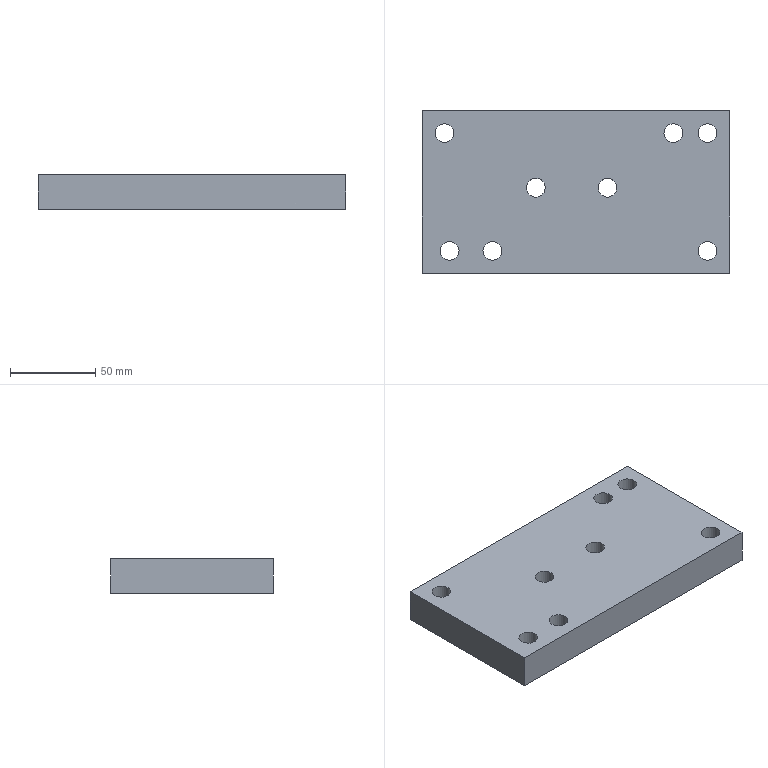Part | STEP file | 111_id2966_x_t | 1 solid | 14 faces | box 180 x 95 x 20 mm | volume 326795 mm3 | cylinder 8 | plane 6 | commonest cylinder face diameters 11 x8
STEP:
#1=CARTESIAN_POINT('',(0.,0.,0.));
#2=DIRECTION('',(0.,0.,1.));
#3=DIRECTION('',(1.,0.,0.));
#4=AXIS2_PLACEMENT_3D('',#1,#2,#3);
#5=CARTESIAN_POINT('',(638.481,67.,105.));
#6=VERTEX_POINT('',#5);
#7=CARTESIAN_POINT('',(627.481,67.,105.));
#8=VERTEX_POINT('',#7);
#9=CARTESIAN_POINT('',(632.981,67.,105.));
#10=DIRECTION('',(0.,0.,1.));
#11=DIRECTION('',(1.,0.,0.));
#12=AXIS2_PLACEMENT_3D('',#9,#10,#11);
#13=CIRCLE('',#12,5.5);
#14=CARTESIAN_POINT('',(657.5,68.,105.));
#15=DIRECTION('',(0.,0.,1.));
#16=DIRECTION('',(-1.,0.,0.));
#17=AXIS2_PLACEMENT_3D('',#14,#15,#16);
#18=PLANE('',#17);
#19=CARTESIAN_POINT('',(24.519,1.));
#20=DIRECTION('',(-1.,0.));
#21=AXIS2_PLACEMENT_2D('',#19,#20);
#22=CIRCLE('',#21,5.5);
#23=(GEOMETRIC_REPRESENTATION_CONTEXT(2)PARAMETRIC_REPRESENTATION_CONTEXT()REPRESENTATION_CONTEXT('',''));
#24=DEFINITIONAL_REPRESENTATION('',(#22),#23);
#25=PCURVE('',#18,#24);
#26=CARTESIAN_POINT('',(632.981,67.,-16.));
#27=DIRECTION('',(0.,0.,1.));
#28=DIRECTION('',(-1.,0.,0.));
#29=AXIS2_PLACEMENT_3D('',#26,#27,#28);
#30=CYLINDRICAL_SURFACE('',#29,5.5);
#31=CARTESIAN_POINT('',(3.142,121.));
#32=DIRECTION('',(1.,0.));
#33=VECTOR('',#32,1.);
#34=LINE('',#31,#33);
#35=(GEOMETRIC_REPRESENTATION_CONTEXT(2)PARAMETRIC_REPRESENTATION_CONTEXT()REPRESENTATION_CONTEXT('',''));
#36=DEFINITIONAL_REPRESENTATION('',(#34),#35);
#37=PCURVE('',#30,#36);
#38=SURFACE_CURVE('',#13,(#25,#37),.PCURVE_S1.);
#39=EDGE_CURVE('',#6,#8,#38,.T.);
#40=ORIENTED_EDGE('',*,*,#39,.F.);
#41=CARTESIAN_POINT('',(632.981,67.,105.));
#42=DIRECTION('',(0.,0.,1.));
#43=DIRECTION('',(1.,0.,0.));
#44=AXIS2_PLACEMENT_3D('',#41,#42,#43);
#45=CIRCLE('',#44,5.5);
#46=CARTESIAN_POINT('',(24.519,1.));
#47=DIRECTION('',(-1.,0.));
#48=AXIS2_PLACEMENT_2D('',#46,#47);
#49=CIRCLE('',#48,5.5);
#50=(GEOMETRIC_REPRESENTATION_CONTEXT(2)PARAMETRIC_REPRESENTATION_CONTEXT()REPRESENTATION_CONTEXT('',''));
#51=DEFINITIONAL_REPRESENTATION('',(#49),#50);
#52=PCURVE('',#18,#51);
#53=CARTESIAN_POINT('',(-3.142,121.));
#54=DIRECTION('',(1.,0.));
#55=VECTOR('',#54,1.);
#56=LINE('',#53,#55);
#57=(GEOMETRIC_REPRESENTATION_CONTEXT(2)PARAMETRIC_REPRESENTATION_CONTEXT()REPRESENTATION_CONTEXT('',''));
#58=DEFINITIONAL_REPRESENTATION('',(#56),#57);
#59=PCURVE('',#30,#58);
#60=SURFACE_CURVE('',#45,(#52,#59),.PCURVE_S1.);
#61=EDGE_CURVE('',#8,#6,#60,.T.);
#62=ORIENTED_EDGE('',*,*,#61,.F.);
#63=EDGE_LOOP('',(#40,#62));
#64=FACE_BOUND('',#63,.T.);
#65=CARTESIAN_POINT('',(680.481,67.,105.));
#66=VERTEX_POINT('',#65);
#67=CARTESIAN_POINT('',(674.981,67.,105.));
#68=DIRECTION('',(0.,0.,1.));
#69=DIRECTION('',(1.,0.,0.));
#70=AXIS2_PLACEMENT_3D('',#67,#68,#69);
#71=CIRCLE('',#70,5.5);
#72=CARTESIAN_POINT('',(-17.481,1.));
#73=DIRECTION('',(-1.,0.));
#74=AXIS2_PLACEMENT_2D('',#72,#73);
#75=CIRCLE('',#74,5.5);
#76=(GEOMETRIC_REPRESENTATION_CONTEXT(2)PARAMETRIC_REPRESENTATION_CONTEXT()REPRESENTATION_CONTEXT('',''));
#77=DEFINITIONAL_REPRESENTATION('',(#75),#76);
#78=PCURVE('',#18,#77);
#79=CARTESIAN_POINT('',(674.981,67.,-16.));
#80=DIRECTION('',(0.,0.,1.));
#81=DIRECTION('',(1.,0.,0.));
#82=AXIS2_PLACEMENT_3D('',#79,#80,#81);
#83=CYLINDRICAL_SURFACE('',#82,5.5);
#84=CARTESIAN_POINT('',(0.,121.));
#85=DIRECTION('',(1.,0.));
#86=VECTOR('',#85,1.);
#87=LINE('',#84,#86);
#88=(GEOMETRIC_REPRESENTATION_CONTEXT(2)PARAMETRIC_REPRESENTATION_CONTEXT()REPRESENTATION_CONTEXT('',''));
#89=DEFINITIONAL_REPRESENTATION('',(#87),#88);
#90=PCURVE('',#83,#89);
#91=SURFACE_CURVE('',#71,(#78,#90),.PCURVE_S1.);
#92=EDGE_CURVE('',#66,#66,#91,.T.);
#93=ORIENTED_EDGE('',*,*,#92,.F.);
#94=EDGE_LOOP('',(#93));
#95=FACE_BOUND('',#94,.T.);
#96=CARTESIAN_POINT('',(613.,30.,105.));
#97=VERTEX_POINT('',#96);
#98=CARTESIAN_POINT('',(607.5,30.,105.));
#99=DIRECTION('',(0.,0.,-1.));
#100=DIRECTION('',(1.,0.,0.));
#101=AXIS2_PLACEMENT_3D('',#98,#99,#100);
#102=CIRCLE('',#101,5.5);
#103=CARTESIAN_POINT('',(44.5,38.));
#104=CARTESIAN_POINT('',(44.5,47.526));
#105=CARTESIAN_POINT('',(52.75,42.763));
#106=CARTESIAN_POINT('',(61.,38.));
#107=CARTESIAN_POINT('',(52.75,33.237));
#108=CARTESIAN_POINT('',(44.5,28.474));
#109=CARTESIAN_POINT('',(44.5,38.));
#110=(BOUNDED_CURVE()B_SPLINE_CURVE(2,(#103,#104,#105,#106,#107,#108,#109),.UNSPECIFIED.,.T.,.F.)B_SPLINE_CURVE_WITH_KNOTS((1,2,2,2,2,1),(-2.094,0.,2.094,4.189,6.283,8.378),.UNSPECIFIED.)CURVE()GEOMETRIC_REPRESENTATION_ITEM()RATIONAL_B_SPLINE_CURVE((1.,0.5,1.,0.5,1.,0.5,1.))REPRESENTATION_ITEM(''));
#111=(GEOMETRIC_REPRESENTATION_CONTEXT(2)PARAMETRIC_REPRESENTATION_CONTEXT()REPRESENTATION_CONTEXT('',''));
#112=DEFINITIONAL_REPRESENTATION('',(#110),#111);
#113=PCURVE('',#18,#112);
#114=CARTESIAN_POINT('',(607.5,30.,90.));
#115=DIRECTION('',(0.,0.,1.));
#116=DIRECTION('',(-1.,0.,0.));
#117=AXIS2_PLACEMENT_3D('',#114,#115,#116);
#118=CYLINDRICAL_SURFACE('',#117,5.5);
#119=CARTESIAN_POINT('',(9.425,15.));
#120=DIRECTION('',(-1.,0.));
#121=VECTOR('',#120,1.);
#122=LINE('',#119,#121);
#123=(GEOMETRIC_REPRESENTATION_CONTEXT(2)PARAMETRIC_REPRESENTATION_CONTEXT()REPRESENTATION_CONTEXT('',''));
#124=DEFINITIONAL_REPRESENTATION('',(#122),#123);
#125=PCURVE('',#118,#124);
#126=SURFACE_CURVE('',#102,(#113,#125),.PCURVE_S1.);
#127=EDGE_CURVE('',#97,#97,#126,.T.);
#128=ORIENTED_EDGE('',*,*,#127,.T.);
#129=EDGE_LOOP('',(#128));
#130=FACE_BOUND('',#129,.T.);
#131=CARTESIAN_POINT('',(739.,99.,105.));
#132=VERTEX_POINT('',#131);
#133=CARTESIAN_POINT('',(733.5,99.,105.));
#134=DIRECTION('',(0.,0.,-1.));
#135=DIRECTION('',(1.,0.,0.));
#136=AXIS2_PLACEMENT_3D('',#133,#134,#135);
#137=CIRCLE('',#136,5.5);
#138=CARTESIAN_POINT('',(-81.5,-31.));
#139=CARTESIAN_POINT('',(-81.5,-21.474));
#140=CARTESIAN_POINT('',(-73.25,-26.237));
#141=CARTESIAN_POINT('',(-65.,-31.));
#142=CARTESIAN_POINT('',(-73.25,-35.763));
#143=CARTESIAN_POINT('',(-81.5,-40.526));
#144=CARTESIAN_POINT('',(-81.5,-31.));
#145=(BOUNDED_CURVE()B_SPLINE_CURVE(2,(#138,#139,#140,#141,#142,#143,#144),.UNSPECIFIED.,.T.,.F.)B_SPLINE_CURVE_WITH_KNOTS((1,2,2,2,2,1),(-2.094,0.,2.094,4.189,6.283,8.378),.UNSPECIFIED.)CURVE()GEOMETRIC_REPRESENTATION_ITEM()RATIONAL_B_SPLINE_CURVE((1.,0.5,1.,0.5,1.,0.5,1.))REPRESENTATION_ITEM(''));
#146=(GEOMETRIC_REPRESENTATION_CONTEXT(2)PARAMETRIC_REPRESENTATION_CONTEXT()REPRESENTATION_CONTEXT('',''));
#147=DEFINITIONAL_REPRESENTATION('',(#145),#146);
#148=PCURVE('',#18,#147);
#149=CARTESIAN_POINT('',(733.5,99.,90.));
#150=DIRECTION('',(0.,0.,1.));
#151=DIRECTION('',(-1.,0.,0.));
#152=AXIS2_PLACEMENT_3D('',#149,#150,#151);
#153=CYLINDRICAL_SURFACE('',#152,5.5);
#154=CARTESIAN_POINT('',(9.425,15.));
#155=DIRECTION('',(-1.,0.));
#156=VECTOR('',#155,1.);
#157=LINE('',#154,#156);
#158=(GEOMETRIC_REPRESENTATION_CONTEXT(2)PARAMETRIC_REPRESENTATION_CONTEXT()REPRESENTATION_CONTEXT('',''));
#159=DEFINITIONAL_REPRESENTATION('',(#157),#158);
#160=PCURVE('',#153,#159);
#161=SURFACE_CURVE('',#137,(#148,#160),.PCURVE_S1.);
#162=EDGE_CURVE('',#132,#132,#161,.T.);
#163=ORIENTED_EDGE('',*,*,#162,.T.);
#164=EDGE_LOOP('',(#163));
#165=FACE_BOUND('',#164,.T.);
#166=CARTESIAN_POINT('',(588.,30.,105.));
#167=VERTEX_POINT('',#166);
#168=CARTESIAN_POINT('',(582.5,30.,105.));
#169=DIRECTION('',(0.,0.,-1.));
#170=DIRECTION('',(1.,0.,0.));
#171=AXIS2_PLACEMENT_3D('',#168,#169,#170);
#172=CIRCLE('',#171,5.5);
#173=CARTESIAN_POINT('',(69.5,38.));
#174=CARTESIAN_POINT('',(69.5,47.526));
#175=CARTESIAN_POINT('',(77.75,42.763));
#176=CARTESIAN_POINT('',(86.,38.));
#177=CARTESIAN_POINT('',(77.75,33.237));
#178=CARTESIAN_POINT('',(69.5,28.474));
#179=CARTESIAN_POINT('',(69.5,38.));
#180=(BOUNDED_CURVE()B_SPLINE_CURVE(2,(#173,#174,#175,#176,#177,#178,#179),.UNSPECIFIED.,.T.,.F.)B_SPLINE_CURVE_WITH_KNOTS((1,2,2,2,2,1),(-2.094,0.,2.094,4.189,6.283,8.378),.UNSPECIFIED.)CURVE()GEOMETRIC_REPRESENTATION_ITEM()RATIONAL_B_SPLINE_CURVE((1.,0.5,1.,0.5,1.,0.5,1.))REPRESENTATION_ITEM(''));
#181=(GEOMETRIC_REPRESENTATION_CONTEXT(2)PARAMETRIC_REPRESENTATION_CONTEXT()REPRESENTATION_CONTEXT('',''));
#182=DEFINITIONAL_REPRESENTATION('',(#180),#181);
#183=PCURVE('',#18,#182);
#184=CARTESIAN_POINT('',(582.5,30.,90.));
#185=DIRECTION('',(0.,0.,1.));
#186=DIRECTION('',(-1.,0.,0.));
#187=AXIS2_PLACEMENT_3D('',#184,#185,#186);
#188=CYLINDRICAL_SURFACE('',#187,5.5);
#189=CARTESIAN_POINT('',(9.425,15.));
#190=DIRECTION('',(-1.,0.));
#191=VECTOR('',#190,1.);
#192=LINE('',#189,#191);
#193=(GEOMETRIC_REPRESENTATION_CONTEXT(2)PARAMETRIC_REPRESENTATION_CONTEXT()REPRESENTATION_CONTEXT('',''));
#194=DEFINITIONAL_REPRESENTATION('',(#192),#193);
#195=PCURVE('',#188,#194);
#196=SURFACE_CURVE('',#172,(#183,#195),.PCURVE_S1.);
#197=EDGE_CURVE('',#167,#167,#196,.T.);
#198=ORIENTED_EDGE('',*,*,#197,.T.);
#199=EDGE_LOOP('',(#198));
#200=FACE_BOUND('',#199,.T.);
#201=CARTESIAN_POINT('',(746.5,17.,105.));
#202=VERTEX_POINT('',#201);
#203=CARTESIAN_POINT('',(566.5,17.,105.));
#204=VERTEX_POINT('',#203);
#205=CARTESIAN_POINT('',(657.5,17.,105.));
#206=DIRECTION('',(-1.,0.,0.));
#207=VECTOR('',#206,1.);
#208=LINE('',#205,#207);
#209=CARTESIAN_POINT('',(0.,51.));
#210=DIRECTION('',(1.,0.));
#211=VECTOR('',#210,1.);
#212=LINE('',#209,#211);
#213=(GEOMETRIC_REPRESENTATION_CONTEXT(2)PARAMETRIC_REPRESENTATION_CONTEXT()REPRESENTATION_CONTEXT('',''));
#214=DEFINITIONAL_REPRESENTATION('',(#212),#213);
#215=PCURVE('',#18,#214);
#216=CARTESIAN_POINT('',(657.5,17.,90.));
#217=DIRECTION('',(0.,-1.,0.));
#218=DIRECTION('',(0.,0.,1.));
#219=AXIS2_PLACEMENT_3D('',#216,#217,#218);
#220=PLANE('',#219);
#221=CARTESIAN_POINT('',(15.,0.));
#222=DIRECTION('',(0.,1.));
#223=VECTOR('',#222,1.);
#224=LINE('',#221,#223);
#225=(GEOMETRIC_REPRESENTATION_CONTEXT(2)PARAMETRIC_REPRESENTATION_CONTEXT()REPRESENTATION_CONTEXT('',''));
#226=DEFINITIONAL_REPRESENTATION('',(#224),#225);
#227=PCURVE('',#220,#226);
#228=SURFACE_CURVE('',#208,(#215,#227),.PCURVE_S1.);
#229=EDGE_CURVE('',#202,#204,#228,.T.);
#230=ORIENTED_EDGE('',*,*,#229,.F.);
#231=CARTESIAN_POINT('',(746.5,112.,105.));
#232=VERTEX_POINT('',#231);
#233=CARTESIAN_POINT('',(746.5,68.,105.));
#234=DIRECTION('',(0.,-1.,0.));
#235=VECTOR('',#234,1.);
#236=LINE('',#233,#235);
#237=CARTESIAN_POINT('',(-89.,0.));
#238=DIRECTION('',(0.,1.));
#239=VECTOR('',#238,1.);
#240=LINE('',#237,#239);
#241=(GEOMETRIC_REPRESENTATION_CONTEXT(2)PARAMETRIC_REPRESENTATION_CONTEXT()REPRESENTATION_CONTEXT('',''));
#242=DEFINITIONAL_REPRESENTATION('',(#240),#241);
#243=PCURVE('',#18,#242);
#244=CARTESIAN_POINT('',(746.5,68.,90.));
#245=DIRECTION('',(1.,0.,0.));
#246=DIRECTION('',(0.,0.,1.));
#247=AXIS2_PLACEMENT_3D('',#244,#245,#246);
#248=PLANE('',#247);
#249=CARTESIAN_POINT('',(15.,0.));
#250=DIRECTION('',(0.,1.));
#251=VECTOR('',#250,1.);
#252=LINE('',#249,#251);
#253=(GEOMETRIC_REPRESENTATION_CONTEXT(2)PARAMETRIC_REPRESENTATION_CONTEXT()REPRESENTATION_CONTEXT('',''));
#254=DEFINITIONAL_REPRESENTATION('',(#252),#253);
#255=PCURVE('',#248,#254);
#256=SURFACE_CURVE('',#236,(#243,#255),.PCURVE_S1.);
#257=EDGE_CURVE('',#232,#202,#256,.T.);
#258=ORIENTED_EDGE('',*,*,#257,.F.);
#259=CARTESIAN_POINT('',(566.5,112.,105.));
#260=VERTEX_POINT('',#259);
#261=CARTESIAN_POINT('',(657.5,112.,105.));
#262=DIRECTION('',(1.,0.,0.));
#263=VECTOR('',#262,1.);
#264=LINE('',#261,#263);
#265=CARTESIAN_POINT('',(0.,-44.));
#266=DIRECTION('',(-1.,0.));
#267=VECTOR('',#266,1.);
#268=LINE('',#265,#267);
#269=(GEOMETRIC_REPRESENTATION_CONTEXT(2)PARAMETRIC_REPRESENTATION_CONTEXT()REPRESENTATION_CONTEXT('',''));
#270=DEFINITIONAL_REPRESENTATION('',(#268),#269);
#271=PCURVE('',#18,#270);
#272=CARTESIAN_POINT('',(657.5,112.,90.));
#273=DIRECTION('',(0.,1.,0.));
#274=DIRECTION('',(0.,0.,-1.));
#275=AXIS2_PLACEMENT_3D('',#272,#273,#274);
#276=PLANE('',#275);
#277=CARTESIAN_POINT('',(-15.,0.));
#278=DIRECTION('',(0.,-1.));
#279=VECTOR('',#278,1.);
#280=LINE('',#277,#279);
#281=(GEOMETRIC_REPRESENTATION_CONTEXT(2)PARAMETRIC_REPRESENTATION_CONTEXT()REPRESENTATION_CONTEXT('',''));
#282=DEFINITIONAL_REPRESENTATION('',(#280),#281);
#283=PCURVE('',#276,#282);
#284=SURFACE_CURVE('',#264,(#271,#283),.PCURVE_S1.);
#285=EDGE_CURVE('',#260,#232,#284,.T.);
#286=ORIENTED_EDGE('',*,*,#285,.F.);
#287=CARTESIAN_POINT('',(566.5,68.,105.));
#288=DIRECTION('',(0.,1.,0.));
#289=VECTOR('',#288,1.);
#290=LINE('',#287,#289);
#291=CARTESIAN_POINT('',(91.,0.));
#292=DIRECTION('',(0.,-1.));
#293=VECTOR('',#292,1.);
#294=LINE('',#291,#293);
#295=(GEOMETRIC_REPRESENTATION_CONTEXT(2)PARAMETRIC_REPRESENTATION_CONTEXT()REPRESENTATION_CONTEXT('',''));
#296=DEFINITIONAL_REPRESENTATION('',(#294),#295);
#297=PCURVE('',#18,#296);
#298=CARTESIAN_POINT('',(566.5,68.,90.));
#299=DIRECTION('',(-1.,0.,0.));
#300=DIRECTION('',(0.,0.,-1.));
#301=AXIS2_PLACEMENT_3D('',#298,#299,#300);
#302=PLANE('',#301);
#303=CARTESIAN_POINT('',(-15.,0.));
#304=DIRECTION('',(0.,-1.));
#305=VECTOR('',#304,1.);
#306=LINE('',#303,#305);
#307=(GEOMETRIC_REPRESENTATION_CONTEXT(2)PARAMETRIC_REPRESENTATION_CONTEXT()REPRESENTATION_CONTEXT('',''));
#308=DEFINITIONAL_REPRESENTATION('',(#306),#307);
#309=PCURVE('',#302,#308);
#310=SURFACE_CURVE('',#290,(#297,#309),.PCURVE_S1.);
#311=EDGE_CURVE('',#204,#260,#310,.T.);
#312=ORIENTED_EDGE('',*,*,#311,.F.);
#313=EDGE_LOOP('',(#230,#258,#286,#312));
#314=FACE_BOUND('',#313,.T.);
#315=CARTESIAN_POINT('',(739.,30.,105.));
#316=VERTEX_POINT('',#315);
#317=CARTESIAN_POINT('',(733.5,30.,105.));
#318=DIRECTION('',(0.,0.,-1.));
#319=DIRECTION('',(1.,0.,0.));
#320=AXIS2_PLACEMENT_3D('',#317,#318,#319);
#321=CIRCLE('',#320,5.5);
#322=CARTESIAN_POINT('',(-81.5,38.));
#323=CARTESIAN_POINT('',(-81.5,47.526));
#324=CARTESIAN_POINT('',(-73.25,42.763));
#325=CARTESIAN_POINT('',(-65.,38.));
#326=CARTESIAN_POINT('',(-73.25,33.237));
#327=CARTESIAN_POINT('',(-81.5,28.474));
#328=CARTESIAN_POINT('',(-81.5,38.));
#329=(BOUNDED_CURVE()B_SPLINE_CURVE(2,(#322,#323,#324,#325,#326,#327,#328),.UNSPECIFIED.,.T.,.F.)B_SPLINE_CURVE_WITH_KNOTS((1,2,2,2,2,1),(-2.094,0.,2.094,4.189,6.283,8.378),.UNSPECIFIED.)CURVE()GEOMETRIC_REPRESENTATION_ITEM()RATIONAL_B_SPLINE_CURVE((1.,0.5,1.,0.5,1.,0.5,1.))REPRESENTATION_ITEM(''));
#330=(GEOMETRIC_REPRESENTATION_CONTEXT(2)PARAMETRIC_REPRESENTATION_CONTEXT()REPRESENTATION_CONTEXT('',''));
#331=DEFINITIONAL_REPRESENTATION('',(#329),#330);
#332=PCURVE('',#18,#331);
#333=CARTESIAN_POINT('',(733.5,30.,90.));
#334=DIRECTION('',(0.,0.,1.));
#335=DIRECTION('',(-1.,0.,0.));
#336=AXIS2_PLACEMENT_3D('',#333,#334,#335);
#337=CYLINDRICAL_SURFACE('',#336,5.5);
#338=CARTESIAN_POINT('',(9.425,15.));
#339=DIRECTION('',(-1.,0.));
#340=VECTOR('',#339,1.);
#341=LINE('',#338,#340);
#342=(GEOMETRIC_REPRESENTATION_CONTEXT(2)PARAMETRIC_REPRESENTATION_CONTEXT()REPRESENTATION_CONTEXT('',''));
#343=DEFINITIONAL_REPRESENTATION('',(#341),#342);
#344=PCURVE('',#337,#343);
#345=SURFACE_CURVE('',#321,(#332,#344),.PCURVE_S1.);
#346=EDGE_CURVE('',#316,#316,#345,.T.);
#347=ORIENTED_EDGE('',*,*,#346,.T.);
#348=EDGE_LOOP('',(#347));
#349=FACE_BOUND('',#348,.T.);
#350=CARTESIAN_POINT('',(585.,99.,105.));
#351=VERTEX_POINT('',#350);
#352=CARTESIAN_POINT('',(579.5,99.,105.));
#353=DIRECTION('',(0.,0.,-1.));
#354=DIRECTION('',(1.,0.,0.));
#355=AXIS2_PLACEMENT_3D('',#352,#353,#354);
#356=CIRCLE('',#355,5.5);
#357=CARTESIAN_POINT('',(72.5,-31.));
#358=CARTESIAN_POINT('',(72.5,-21.474));
#359=CARTESIAN_POINT('',(80.75,-26.237));
#360=CARTESIAN_POINT('',(89.,-31.));
#361=CARTESIAN_POINT('',(80.75,-35.763));
#362=CARTESIAN_POINT('',(72.5,-40.526));
#363=CARTESIAN_POINT('',(72.5,-31.));
#364=(BOUNDED_CURVE()B_SPLINE_CURVE(2,(#357,#358,#359,#360,#361,#362,#363),.UNSPECIFIED.,.T.,.F.)B_SPLINE_CURVE_WITH_KNOTS((1,2,2,2,2,1),(-2.094,0.,2.094,4.189,6.283,8.378),.UNSPECIFIED.)CURVE()GEOMETRIC_REPRESENTATION_ITEM()RATIONAL_B_SPLINE_CURVE((1.,0.5,1.,0.5,1.,0.5,1.))REPRESENTATION_ITEM(''));
#365=(GEOMETRIC_REPRESENTATION_CONTEXT(2)PARAMETRIC_REPRESENTATION_CONTEXT()REPRESENTATION_CONTEXT('',''));
#366=DEFINITIONAL_REPRESENTATION('',(#364),#365);
#367=PCURVE('',#18,#366);
#368=CARTESIAN_POINT('',(579.5,99.,90.));
#369=DIRECTION('',(0.,0.,1.));
#370=DIRECTION('',(-1.,0.,0.));
#371=AXIS2_PLACEMENT_3D('',#368,#369,#370);
#372=CYLINDRICAL_SURFACE('',#371,5.5);
#373=CARTESIAN_POINT('',(9.425,15.));
#374=DIRECTION('',(-1.,0.));
#375=VECTOR('',#374,1.);
#376=LINE('',#373,#375);
#377=(GEOMETRIC_REPRESENTATION_CONTEXT(2)PARAMETRIC_REPRESENTATION_CONTEXT()REPRESENTATION_CONTEXT('',''));
#378=DEFINITIONAL_REPRESENTATION('',(#376),#377);
#379=PCURVE('',#372,#378);
#380=SURFACE_CURVE('',#356,(#367,#379),.PCURVE_S1.);
#381=EDGE_CURVE('',#351,#351,#380,.T.);
#382=ORIENTED_EDGE('',*,*,#381,.T.);
#383=EDGE_LOOP('',(#382));
#384=FACE_BOUND('',#383,.T.);
#385=CARTESIAN_POINT('',(719.,99.,105.));
#386=VERTEX_POINT('',#385);
#387=CARTESIAN_POINT('',(713.5,99.,105.));
#388=DIRECTION('',(0.,0.,-1.));
#389=DIRECTION('',(1.,0.,0.));
#390=AXIS2_PLACEMENT_3D('',#387,#388,#389);
#391=CIRCLE('',#390,5.5);
#392=CARTESIAN_POINT('',(-61.5,-31.));
#393=CARTESIAN_POINT('',(-61.5,-21.474));
#394=CARTESIAN_POINT('',(-53.25,-26.237));
#395=CARTESIAN_POINT('',(-45.,-31.));
#396=CARTESIAN_POINT('',(-53.25,-35.763));
#397=CARTESIAN_POINT('',(-61.5,-40.526));
#398=CARTESIAN_POINT('',(-61.5,-31.));
#399=(BOUNDED_CURVE()B_SPLINE_CURVE(2,(#392,#393,#394,#395,#396,#397,#398),.UNSPECIFIED.,.T.,.F.)B_SPLINE_CURVE_WITH_KNOTS((1,2,2,2,2,1),(-2.094,0.,2.094,4.189,6.283,8.378),.UNSPECIFIED.)CURVE()GEOMETRIC_REPRESENTATION_ITEM()RATIONAL_B_SPLINE_CURVE((1.,0.5,1.,0.5,1.,0.5,1.))REPRESENTATION_ITEM(''));
#400=(GEOMETRIC_REPRESENTATION_CONTEXT(2)PARAMETRIC_REPRESENTATION_CONTEXT()REPRESENTATION_CONTEXT('',''));
#401=DEFINITIONAL_REPRESENTATION('',(#399),#400);
#402=PCURVE('',#18,#401);
#403=CARTESIAN_POINT('',(713.5,99.,90.));
#404=DIRECTION('',(0.,0.,1.));
#405=DIRECTION('',(-1.,0.,0.));
#406=AXIS2_PLACEMENT_3D('',#403,#404,#405);
#407=CYLINDRICAL_SURFACE('',#406,5.5);
#408=CARTESIAN_POINT('',(9.425,15.));
#409=DIRECTION('',(-1.,0.));
#410=VECTOR('',#409,1.);
#411=LINE('',#408,#410);
#412=(GEOMETRIC_REPRESENTATION_CONTEXT(2)PARAMETRIC_REPRESENTATION_CONTEXT()REPRESENTATION_CONTEXT('',''));
#413=DEFINITIONAL_REPRESENTATION('',(#411),#412);
#414=PCURVE('',#407,#413);
#415=SURFACE_CURVE('',#391,(#402,#414),.PCURVE_S1.);
#416=EDGE_CURVE('',#386,#386,#415,.T.);
#417=ORIENTED_EDGE('',*,*,#416,.T.);
#418=EDGE_LOOP('',(#417));
#419=FACE_BOUND('',#418,.T.);
#420=ADVANCED_FACE('',(#64,#95,#130,#165,#200,#314,#349,#384,#419),#18,.T.);
#421=CARTESIAN_POINT('',(627.481,67.,85.));
#422=VERTEX_POINT('',#421);
#423=CARTESIAN_POINT('',(632.981,67.,85.));
#424=DIRECTION('',(0.,0.,-1.));
#425=DIRECTION('',(-1.,0.,0.));
#426=AXIS2_PLACEMENT_3D('',#423,#424,#425);
#427=CIRCLE('',#426,5.5);
#428=CARTESIAN_POINT('',(657.5,68.,85.));
#429=DIRECTION('',(0.,0.,-1.));
#430=DIRECTION('',(1.,0.,0.));
#431=AXIS2_PLACEMENT_3D('',#428,#429,#430);
#432=PLANE('',#431);
#433=CARTESIAN_POINT('',(-24.519,1.));
#434=DIRECTION('',(-1.,0.));
#435=AXIS2_PLACEMENT_2D('',#433,#434);
#436=CIRCLE('',#435,5.5);
#437=(GEOMETRIC_REPRESENTATION_CONTEXT(2)PARAMETRIC_REPRESENTATION_CONTEXT()REPRESENTATION_CONTEXT('',''));
#438=DEFINITIONAL_REPRESENTATION('',(#436),#437);
#439=PCURVE('',#432,#438);
#440=CARTESIAN_POINT('',(6.283,101.));
#441=DIRECTION('',(-1.,0.));
#442=VECTOR('',#441,1.);
#443=LINE('',#440,#442);
#444=(GEOMETRIC_REPRESENTATION_CONTEXT(2)PARAMETRIC_REPRESENTATION_CONTEXT()REPRESENTATION_CONTEXT('',''));
#445=DEFINITIONAL_REPRESENTATION('',(#443),#444);
#446=PCURVE('',#30,#445);
#447=SURFACE_CURVE('',#427,(#439,#446),.PCURVE_S1.);
#448=EDGE_CURVE('',#422,#422,#447,.T.);
#449=ORIENTED_EDGE('',*,*,#448,.F.);
#450=EDGE_LOOP('',(#449));
#451=FACE_BOUND('',#450,.T.);
#452=CARTESIAN_POINT('',(669.481,67.,85.));
#453=VERTEX_POINT('',#452);
#454=CARTESIAN_POINT('',(680.481,67.,85.));
#455=VERTEX_POINT('',#454);
#456=CARTESIAN_POINT('',(674.981,67.,85.));
#457=DIRECTION('',(0.,0.,-1.));
#458=DIRECTION('',(-1.,0.,0.));
#459=AXIS2_PLACEMENT_3D('',#456,#457,#458);
#460=CIRCLE('',#459,5.5);
#461=CARTESIAN_POINT('',(17.481,1.));
#462=DIRECTION('',(-1.,0.));
#463=AXIS2_PLACEMENT_2D('',#461,#462);
#464=CIRCLE('',#463,5.5);
#465=(GEOMETRIC_REPRESENTATION_CONTEXT(2)PARAMETRIC_REPRESENTATION_CONTEXT()REPRESENTATION_CONTEXT('',''));
#466=DEFINITIONAL_REPRESENTATION('',(#464),#465);
#467=PCURVE('',#432,#466);
#468=CARTESIAN_POINT('',(3.142,101.));
#469=DIRECTION('',(-1.,0.));
#470=VECTOR('',#469,1.);
#471=LINE('',#468,#470);
#472=(GEOMETRIC_REPRESENTATION_CONTEXT(2)PARAMETRIC_REPRESENTATION_CONTEXT()REPRESENTATION_CONTEXT('',''));
#473=DEFINITIONAL_REPRESENTATION('',(#471),#472);
#474=PCURVE('',#83,#473);
#475=SURFACE_CURVE('',#460,(#467,#474),.PCURVE_S1.);
#476=EDGE_CURVE('',#453,#455,#475,.T.);
#477=ORIENTED_EDGE('',*,*,#476,.F.);
#478=CARTESIAN_POINT('',(674.981,67.,85.));
#479=DIRECTION('',(0.,0.,-1.));
#480=DIRECTION('',(-1.,0.,0.));
#481=AXIS2_PLACEMENT_3D('',#478,#479,#480);
#482=CIRCLE('',#481,5.5);
#483=CARTESIAN_POINT('',(17.481,1.));
#484=DIRECTION('',(-1.,0.));
#485=AXIS2_PLACEMENT_2D('',#483,#484);
#486=CIRCLE('',#485,5.5);
#487=(GEOMETRIC_REPRESENTATION_CONTEXT(2)PARAMETRIC_REPRESENTATION_CONTEXT()REPRESENTATION_CONTEXT('',''));
#488=DEFINITIONAL_REPRESENTATION('',(#486),#487);
#489=PCURVE('',#432,#488);
#490=CARTESIAN_POINT('',(9.425,101.));
#491=DIRECTION('',(-1.,0.));
#492=VECTOR('',#491,1.);
#493=LINE('',#490,#492);
#494=(GEOMETRIC_REPRESENTATION_CONTEXT(2)PARAMETRIC_REPRESENTATION_CONTEXT()REPRESENTATION_CONTEXT('',''));
#495=DEFINITIONAL_REPRESENTATION('',(#493),#494);
#496=PCURVE('',#83,#495);
#497=SURFACE_CURVE('',#482,(#489,#496),.PCURVE_S1.);
#498=EDGE_CURVE('',#455,#453,#497,.T.);
#499=ORIENTED_EDGE('',*,*,#498,.F.);
#500=EDGE_LOOP('',(#477,#499));
#501=FACE_BOUND('',#500,.T.);
#502=CARTESIAN_POINT('',(613.,30.,85.));
#503=VERTEX_POINT('',#502);
#504=CARTESIAN_POINT('',(607.5,30.,85.));
#505=DIRECTION('',(0.,0.,1.));
#506=DIRECTION('',(-1.,0.,0.));
#507=AXIS2_PLACEMENT_3D('',#504,#505,#506);
#508=CIRCLE('',#507,5.5);
#509=CARTESIAN_POINT('',(-55.5,38.));
#510=CARTESIAN_POINT('',(-55.5,47.526));
#511=CARTESIAN_POINT('',(-47.25,42.763));
#512=CARTESIAN_POINT('',(-39.,38.));
#513=CARTESIAN_POINT('',(-47.25,33.237));
#514=CARTESIAN_POINT('',(-55.5,28.474));
#515=CARTESIAN_POINT('',(-55.5,38.));
#516=(BOUNDED_CURVE()B_SPLINE_CURVE(2,(#509,#510,#511,#512,#513,#514,#515),.UNSPECIFIED.,.T.,.F.)B_SPLINE_CURVE_WITH_KNOTS((1,2,2,2,2,1),(-2.094,0.,2.094,4.189,6.283,8.378),.UNSPECIFIED.)CURVE()GEOMETRIC_REPRESENTATION_ITEM()RATIONAL_B_SPLINE_CURVE((1.,0.5,1.,0.5,1.,0.5,1.))REPRESENTATION_ITEM(''));
#517=(GEOMETRIC_REPRESENTATION_CONTEXT(2)PARAMETRIC_REPRESENTATION_CONTEXT()REPRESENTATION_CONTEXT('',''));
#518=DEFINITIONAL_REPRESENTATION('',(#516),#517);
#519=PCURVE('',#432,#518);
#520=CARTESIAN_POINT('',(0.,-5.));
#521=DIRECTION('',(1.,0.));
#522=VECTOR('',#521,1.);
#523=LINE('',#520,#522);
#524=(GEOMETRIC_REPRESENTATION_CONTEXT(2)PARAMETRIC_REPRESENTATION_CONTEXT()REPRESENTATION_CONTEXT('',''));
#525=DEFINITIONAL_REPRESENTATION('',(#523),#524);
#526=PCURVE('',#118,#525);
#527=SURFACE_CURVE('',#508,(#519,#526),.PCURVE_S1.);
#528=EDGE_CURVE('',#503,#503,#527,.T.);
#529=ORIENTED_EDGE('',*,*,#528,.T.);
#530=EDGE_LOOP('',(#529));
#531=FACE_BOUND('',#530,.T.);
#532=CARTESIAN_POINT('',(739.,99.,85.));
#533=VERTEX_POINT('',#532);
#534=CARTESIAN_POINT('',(733.5,99.,85.));
#535=DIRECTION('',(0.,0.,1.));
#536=DIRECTION('',(-1.,0.,0.));
#537=AXIS2_PLACEMENT_3D('',#534,#535,#536);
#538=CIRCLE('',#537,5.5);
#539=CARTESIAN_POINT('',(70.5,-31.));
#540=CARTESIAN_POINT('',(70.5,-21.474));
#541=CARTESIAN_POINT('',(78.75,-26.237));
#542=CARTESIAN_POINT('',(87.,-31.));
#543=CARTESIAN_POINT('',(78.75,-35.763));
#544=CARTESIAN_POINT('',(70.5,-40.526));
#545=CARTESIAN_POINT('',(70.5,-31.));
#546=(BOUNDED_CURVE()B_SPLINE_CURVE(2,(#539,#540,#541,#542,#543,#544,#545),.UNSPECIFIED.,.T.,.F.)B_SPLINE_CURVE_WITH_KNOTS((1,2,2,2,2,1),(-2.094,0.,2.094,4.189,6.283,8.378),.UNSPECIFIED.)CURVE()GEOMETRIC_REPRESENTATION_ITEM()RATIONAL_B_SPLINE_CURVE((1.,0.5,1.,0.5,1.,0.5,1.))REPRESENTATION_ITEM(''));
#547=(GEOMETRIC_REPRESENTATION_CONTEXT(2)PARAMETRIC_REPRESENTATION_CONTEXT()REPRESENTATION_CONTEXT('',''));
#548=DEFINITIONAL_REPRESENTATION('',(#546),#547);
#549=PCURVE('',#432,#548);
#550=CARTESIAN_POINT('',(0.,-5.));
#551=DIRECTION('',(1.,0.));
#552=VECTOR('',#551,1.);
#553=LINE('',#550,#552);
#554=(GEOMETRIC_REPRESENTATION_CONTEXT(2)PARAMETRIC_REPRESENTATION_CONTEXT()REPRESENTATION_CONTEXT('',''));
#555=DEFINITIONAL_REPRESENTATION('',(#553),#554);
#556=PCURVE('',#153,#555);
#557=SURFACE_CURVE('',#538,(#549,#556),.PCURVE_S1.);
#558=EDGE_CURVE('',#533,#533,#557,.T.);
#559=ORIENTED_EDGE('',*,*,#558,.T.);
#560=EDGE_LOOP('',(#559));
#561=FACE_BOUND('',#560,.T.);
#562=CARTESIAN_POINT('',(588.,30.,85.));
#563=VERTEX_POINT('',#562);
#564=CARTESIAN_POINT('',(582.5,30.,85.));
#565=DIRECTION('',(0.,0.,1.));
#566=DIRECTION('',(-1.,0.,0.));
#567=AXIS2_PLACEMENT_3D('',#564,#565,#566);
#568=CIRCLE('',#567,5.5);
#569=CARTESIAN_POINT('',(-80.5,38.));
#570=CARTESIAN_POINT('',(-80.5,47.526));
#571=CARTESIAN_POINT('',(-72.25,42.763));
#572=CARTESIAN_POINT('',(-64.,38.));
#573=CARTESIAN_POINT('',(-72.25,33.237));
#574=CARTESIAN_POINT('',(-80.5,28.474));
#575=CARTESIAN_POINT('',(-80.5,38.));
#576=(BOUNDED_CURVE()B_SPLINE_CURVE(2,(#569,#570,#571,#572,#573,#574,#575),.UNSPECIFIED.,.T.,.F.)B_SPLINE_CURVE_WITH_KNOTS((1,2,2,2,2,1),(-2.094,0.,2.094,4.189,6.283,8.378),.UNSPECIFIED.)CURVE()GEOMETRIC_REPRESENTATION_ITEM()RATIONAL_B_SPLINE_CURVE((1.,0.5,1.,0.5,1.,0.5,1.))REPRESENTATION_ITEM(''));
#577=(GEOMETRIC_REPRESENTATION_CONTEXT(2)PARAMETRIC_REPRESENTATION_CONTEXT()REPRESENTATION_CONTEXT('',''));
#578=DEFINITIONAL_REPRESENTATION('',(#576),#577);
#579=PCURVE('',#432,#578);
#580=CARTESIAN_POINT('',(0.,-5.));
#581=DIRECTION('',(1.,0.));
#582=VECTOR('',#581,1.);
#583=LINE('',#580,#582);
#584=(GEOMETRIC_REPRESENTATION_CONTEXT(2)PARAMETRIC_REPRESENTATION_CONTEXT()REPRESENTATION_CONTEXT('',''));
#585=DEFINITIONAL_REPRESENTATION('',(#583),#584);
#586=PCURVE('',#188,#585);
#587=SURFACE_CURVE('',#568,(#579,#586),.PCURVE_S1.);
#588=EDGE_CURVE('',#563,#563,#587,.T.);
#589=ORIENTED_EDGE('',*,*,#588,.T.);
#590=EDGE_LOOP('',(#589));
#591=FACE_BOUND('',#590,.T.);
#592=CARTESIAN_POINT('',(746.5,17.,85.));
#593=VERTEX_POINT('',#592);
#594=CARTESIAN_POINT('',(746.5,112.,85.));
#595=VERTEX_POINT('',#594);
#596=CARTESIAN_POINT('',(746.5,68.,85.));
#597=DIRECTION('',(0.,1.,0.));
#598=VECTOR('',#597,1.);
#599=LINE('',#596,#598);
#600=CARTESIAN_POINT('',(89.,0.));
#601=DIRECTION('',(0.,-1.));
#602=VECTOR('',#601,1.);
#603=LINE('',#600,#602);
#604=(GEOMETRIC_REPRESENTATION_CONTEXT(2)PARAMETRIC_REPRESENTATION_CONTEXT()REPRESENTATION_CONTEXT('',''));
#605=DEFINITIONAL_REPRESENTATION('',(#603),#604);
#606=PCURVE('',#432,#605);
#607=CARTESIAN_POINT('',(-5.,0.));
#608=DIRECTION('',(0.,-1.));
#609=VECTOR('',#608,1.);
#610=LINE('',#607,#609);
#611=(GEOMETRIC_REPRESENTATION_CONTEXT(2)PARAMETRIC_REPRESENTATION_CONTEXT()REPRESENTATION_CONTEXT('',''));
#612=DEFINITIONAL_REPRESENTATION('',(#610),#611);
#613=PCURVE('',#248,#612);
#614=SURFACE_CURVE('',#599,(#606,#613),.PCURVE_S1.);
#615=EDGE_CURVE('',#593,#595,#614,.T.);
#616=ORIENTED_EDGE('',*,*,#615,.F.);
#617=CARTESIAN_POINT('',(566.5,17.,85.));
#618=VERTEX_POINT('',#617);
#619=CARTESIAN_POINT('',(657.5,17.,85.));
#620=DIRECTION('',(1.,0.,0.));
#621=VECTOR('',#620,1.);
#622=LINE('',#619,#621);
#623=CARTESIAN_POINT('',(0.,51.));
#624=DIRECTION('',(1.,0.));
#625=VECTOR('',#624,1.);
#626=LINE('',#623,#625);
#627=(GEOMETRIC_REPRESENTATION_CONTEXT(2)PARAMETRIC_REPRESENTATION_CONTEXT()REPRESENTATION_CONTEXT('',''));
#628=DEFINITIONAL_REPRESENTATION('',(#626),#627);
#629=PCURVE('',#432,#628);
#630=CARTESIAN_POINT('',(-5.,0.));
#631=DIRECTION('',(0.,-1.));
#632=VECTOR('',#631,1.);
#633=LINE('',#630,#632);
#634=(GEOMETRIC_REPRESENTATION_CONTEXT(2)PARAMETRIC_REPRESENTATION_CONTEXT()REPRESENTATION_CONTEXT('',''));
#635=DEFINITIONAL_REPRESENTATION('',(#633),#634);
#636=PCURVE('',#220,#635);
#637=SURFACE_CURVE('',#622,(#629,#636),.PCURVE_S1.);
#638=EDGE_CURVE('',#618,#593,#637,.T.);
#639=ORIENTED_EDGE('',*,*,#638,.F.);
#640=CARTESIAN_POINT('',(566.5,112.,85.));
#641=VERTEX_POINT('',#640);
#642=CARTESIAN_POINT('',(566.5,68.,85.));
#643=DIRECTION('',(0.,-1.,0.));
#644=VECTOR('',#643,1.);
#645=LINE('',#642,#644);
#646=CARTESIAN_POINT('',(-91.,0.));
#647=DIRECTION('',(0.,1.));
#648=VECTOR('',#647,1.);
#649=LINE('',#646,#648);
#650=(GEOMETRIC_REPRESENTATION_CONTEXT(2)PARAMETRIC_REPRESENTATION_CONTEXT()REPRESENTATION_CONTEXT('',''));
#651=DEFINITIONAL_REPRESENTATION('',(#649),#650);
#652=PCURVE('',#432,#651);
#653=CARTESIAN_POINT('',(5.,0.));
#654=DIRECTION('',(0.,1.));
#655=VECTOR('',#654,1.);
#656=LINE('',#653,#655);
#657=(GEOMETRIC_REPRESENTATION_CONTEXT(2)PARAMETRIC_REPRESENTATION_CONTEXT()REPRESENTATION_CONTEXT('',''));
#658=DEFINITIONAL_REPRESENTATION('',(#656),#657);
#659=PCURVE('',#302,#658);
#660=SURFACE_CURVE('',#645,(#652,#659),.PCURVE_S1.);
#661=EDGE_CURVE('',#641,#618,#660,.T.);
#662=ORIENTED_EDGE('',*,*,#661,.F.);
#663=CARTESIAN_POINT('',(657.5,112.,85.));
#664=DIRECTION('',(-1.,0.,0.));
#665=VECTOR('',#664,1.);
#666=LINE('',#663,#665);
#667=CARTESIAN_POINT('',(0.,-44.));
#668=DIRECTION('',(-1.,0.));
#669=VECTOR('',#668,1.);
#670=LINE('',#667,#669);
#671=(GEOMETRIC_REPRESENTATION_CONTEXT(2)PARAMETRIC_REPRESENTATION_CONTEXT()REPRESENTATION_CONTEXT('',''));
#672=DEFINITIONAL_REPRESENTATION('',(#670),#671);
#673=PCURVE('',#432,#672);
#674=CARTESIAN_POINT('',(5.,0.));
#675=DIRECTION('',(0.,1.));
#676=VECTOR('',#675,1.);
#677=LINE('',#674,#676);
#678=(GEOMETRIC_REPRESENTATION_CONTEXT(2)PARAMETRIC_REPRESENTATION_CONTEXT()REPRESENTATION_CONTEXT('',''));
#679=DEFINITIONAL_REPRESENTATION('',(#677),#678);
#680=PCURVE('',#276,#679);
#681=SURFACE_CURVE('',#666,(#673,#680),.PCURVE_S1.);
#682=EDGE_CURVE('',#595,#641,#681,.T.);
#683=ORIENTED_EDGE('',*,*,#682,.F.);
#684=EDGE_LOOP('',(#616,#639,#662,#683));
#685=FACE_BOUND('',#684,.T.);
#686=CARTESIAN_POINT('',(739.,30.,85.));
#687=VERTEX_POINT('',#686);
#688=CARTESIAN_POINT('',(733.5,30.,85.));
#689=DIRECTION('',(0.,0.,1.));
#690=DIRECTION('',(-1.,0.,0.));
#691=AXIS2_PLACEMENT_3D('',#688,#689,#690);
#692=CIRCLE('',#691,5.5);
#693=CARTESIAN_POINT('',(70.5,38.));
#694=CARTESIAN_POINT('',(70.5,47.526));
#695=CARTESIAN_POINT('',(78.75,42.763));
#696=CARTESIAN_POINT('',(87.,38.));
#697=CARTESIAN_POINT('',(78.75,33.237));
#698=CARTESIAN_POINT('',(70.5,28.474));
#699=CARTESIAN_POINT('',(70.5,38.));
#700=(BOUNDED_CURVE()B_SPLINE_CURVE(2,(#693,#694,#695,#696,#697,#698,#699),.UNSPECIFIED.,.T.,.F.)B_SPLINE_CURVE_WITH_KNOTS((1,2,2,2,2,1),(-2.094,0.,2.094,4.189,6.283,8.378),.UNSPECIFIED.)CURVE()GEOMETRIC_REPRESENTATION_ITEM()RATIONAL_B_SPLINE_CURVE((1.,0.5,1.,0.5,1.,0.5,1.))REPRESENTATION_ITEM(''));
#701=(GEOMETRIC_REPRESENTATION_CONTEXT(2)PARAMETRIC_REPRESENTATION_CONTEXT()REPRESENTATION_CONTEXT('',''));
#702=DEFINITIONAL_REPRESENTATION('',(#700),#701);
#703=PCURVE('',#432,#702);
#704=CARTESIAN_POINT('',(0.,-5.));
#705=DIRECTION('',(1.,0.));
#706=VECTOR('',#705,1.);
#707=LINE('',#704,#706);
#708=(GEOMETRIC_REPRESENTATION_CONTEXT(2)PARAMETRIC_REPRESENTATION_CONTEXT()REPRESENTATION_CONTEXT('',''));
#709=DEFINITIONAL_REPRESENTATION('',(#707),#708);
#710=PCURVE('',#337,#709);
#711=SURFACE_CURVE('',#692,(#703,#710),.PCURVE_S1.);
#712=EDGE_CURVE('',#687,#687,#711,.T.);
#713=ORIENTED_EDGE('',*,*,#712,.T.);
#714=EDGE_LOOP('',(#713));
#715=FACE_BOUND('',#714,.T.);
#716=CARTESIAN_POINT('',(585.,99.,85.));
#717=VERTEX_POINT('',#716);
#718=CARTESIAN_POINT('',(579.5,99.,85.));
#719=DIRECTION('',(0.,0.,1.));
#720=DIRECTION('',(-1.,0.,0.));
#721=AXIS2_PLACEMENT_3D('',#718,#719,#720);
#722=CIRCLE('',#721,5.5);
#723=CARTESIAN_POINT('',(-83.5,-31.));
#724=CARTESIAN_POINT('',(-83.5,-21.474));
#725=CARTESIAN_POINT('',(-75.25,-26.237));
#726=CARTESIAN_POINT('',(-67.,-31.));
#727=CARTESIAN_POINT('',(-75.25,-35.763));
#728=CARTESIAN_POINT('',(-83.5,-40.526));
#729=CARTESIAN_POINT('',(-83.5,-31.));
#730=(BOUNDED_CURVE()B_SPLINE_CURVE(2,(#723,#724,#725,#726,#727,#728,#729),.UNSPECIFIED.,.T.,.F.)B_SPLINE_CURVE_WITH_KNOTS((1,2,2,2,2,1),(-2.094,0.,2.094,4.189,6.283,8.378),.UNSPECIFIED.)CURVE()GEOMETRIC_REPRESENTATION_ITEM()RATIONAL_B_SPLINE_CURVE((1.,0.5,1.,0.5,1.,0.5,1.))REPRESENTATION_ITEM(''));
#731=(GEOMETRIC_REPRESENTATION_CONTEXT(2)PARAMETRIC_REPRESENTATION_CONTEXT()REPRESENTATION_CONTEXT('',''));
#732=DEFINITIONAL_REPRESENTATION('',(#730),#731);
#733=PCURVE('',#432,#732);
#734=CARTESIAN_POINT('',(0.,-5.));
#735=DIRECTION('',(1.,0.));
#736=VECTOR('',#735,1.);
#737=LINE('',#734,#736);
#738=(GEOMETRIC_REPRESENTATION_CONTEXT(2)PARAMETRIC_REPRESENTATION_CONTEXT()REPRESENTATION_CONTEXT('',''));
#739=DEFINITIONAL_REPRESENTATION('',(#737),#738);
#740=PCURVE('',#372,#739);
#741=SURFACE_CURVE('',#722,(#733,#740),.PCURVE_S1.);
#742=EDGE_CURVE('',#717,#717,#741,.T.);
#743=ORIENTED_EDGE('',*,*,#742,.T.);
#744=EDGE_LOOP('',(#743));
#745=FACE_BOUND('',#744,.T.);
#746=CARTESIAN_POINT('',(719.,99.,85.));
#747=VERTEX_POINT('',#746);
#748=CARTESIAN_POINT('',(713.5,99.,85.));
#749=DIRECTION('',(0.,0.,1.));
#750=DIRECTION('',(-1.,0.,0.));
#751=AXIS2_PLACEMENT_3D('',#748,#749,#750);
#752=CIRCLE('',#751,5.5);
#753=CARTESIAN_POINT('',(50.5,-31.));
#754=CARTESIAN_POINT('',(50.5,-21.474));
#755=CARTESIAN_POINT('',(58.75,-26.237));
#756=CARTESIAN_POINT('',(67.,-31.));
#757=CARTESIAN_POINT('',(58.75,-35.763));
#758=CARTESIAN_POINT('',(50.5,-40.526));
#759=CARTESIAN_POINT('',(50.5,-31.));
#760=(BOUNDED_CURVE()B_SPLINE_CURVE(2,(#753,#754,#755,#756,#757,#758,#759),.UNSPECIFIED.,.T.,.F.)B_SPLINE_CURVE_WITH_KNOTS((1,2,2,2,2,1),(-2.094,0.,2.094,4.189,6.283,8.378),.UNSPECIFIED.)CURVE()GEOMETRIC_REPRESENTATION_ITEM()RATIONAL_B_SPLINE_CURVE((1.,0.5,1.,0.5,1.,0.5,1.))REPRESENTATION_ITEM(''));
#761=(GEOMETRIC_REPRESENTATION_CONTEXT(2)PARAMETRIC_REPRESENTATION_CONTEXT()REPRESENTATION_CONTEXT('',''));
#762=DEFINITIONAL_REPRESENTATION('',(#760),#761);
#763=PCURVE('',#432,#762);
#764=CARTESIAN_POINT('',(0.,-5.));
#765=DIRECTION('',(1.,0.));
#766=VECTOR('',#765,1.);
#767=LINE('',#764,#766);
#768=(GEOMETRIC_REPRESENTATION_CONTEXT(2)PARAMETRIC_REPRESENTATION_CONTEXT()REPRESENTATION_CONTEXT('',''));
#769=DEFINITIONAL_REPRESENTATION('',(#767),#768);
#770=PCURVE('',#407,#769);
#771=SURFACE_CURVE('',#752,(#763,#770),.PCURVE_S1.);
#772=EDGE_CURVE('',#747,#747,#771,.T.);
#773=ORIENTED_EDGE('',*,*,#772,.T.);
#774=EDGE_LOOP('',(#773));
#775=FACE_BOUND('',#774,.T.);
#776=ADVANCED_FACE('',(#451,#501,#531,#561,#591,#685,#715,#745,#775),#432,.T.);
#777=CARTESIAN_POINT('',(746.5,17.,90.));
#778=DIRECTION('',(0.,0.,1.));
#779=VECTOR('',#778,1.);
#780=LINE('',#777,#779);
#781=CARTESIAN_POINT('',(0.,-89.));
#782=DIRECTION('',(1.,0.));
#783=VECTOR('',#782,1.);
#784=LINE('',#781,#783);
#785=(GEOMETRIC_REPRESENTATION_CONTEXT(2)PARAMETRIC_REPRESENTATION_CONTEXT()REPRESENTATION_CONTEXT('',''));
#786=DEFINITIONAL_REPRESENTATION('',(#784),#785);
#787=PCURVE('',#220,#786);
#788=CARTESIAN_POINT('',(0.,51.));
#789=DIRECTION('',(1.,0.));
#790=VECTOR('',#789,1.);
#791=LINE('',#788,#790);
#792=(GEOMETRIC_REPRESENTATION_CONTEXT(2)PARAMETRIC_REPRESENTATION_CONTEXT()REPRESENTATION_CONTEXT('',''));
#793=DEFINITIONAL_REPRESENTATION('',(#791),#792);
#794=PCURVE('',#248,#793);
#795=SURFACE_CURVE('',#780,(#787,#794),.PCURVE_S1.);
#796=EDGE_CURVE('',#593,#202,#795,.T.);
#797=ORIENTED_EDGE('',*,*,#796,.T.);
#798=ORIENTED_EDGE('',*,*,#229,.T.);
#799=CARTESIAN_POINT('',(566.5,17.,90.));
#800=DIRECTION('',(0.,0.,1.));
#801=VECTOR('',#800,1.);
#802=LINE('',#799,#801);
#803=CARTESIAN_POINT('',(0.,91.));
#804=DIRECTION('',(1.,0.));
#805=VECTOR('',#804,1.);
#806=LINE('',#803,#805);
#807=(GEOMETRIC_REPRESENTATION_CONTEXT(2)PARAMETRIC_REPRESENTATION_CONTEXT()REPRESENTATION_CONTEXT('',''));
#808=DEFINITIONAL_REPRESENTATION('',(#806),#807);
#809=PCURVE('',#220,#808);
#810=CARTESIAN_POINT('',(0.,51.));
#811=DIRECTION('',(-1.,0.));
#812=VECTOR('',#811,1.);
#813=LINE('',#810,#812);
#814=(GEOMETRIC_REPRESENTATION_CONTEXT(2)PARAMETRIC_REPRESENTATION_CONTEXT()REPRESENTATION_CONTEXT('',''));
#815=DEFINITIONAL_REPRESENTATION('',(#813),#814);
#816=PCURVE('',#302,#815);
#817=SURFACE_CURVE('',#802,(#809,#816),.PCURVE_S1.);
#818=EDGE_CURVE('',#618,#204,#817,.T.);
#819=ORIENTED_EDGE('',*,*,#818,.F.);
#820=ORIENTED_EDGE('',*,*,#638,.T.);
#821=EDGE_LOOP('',(#797,#798,#819,#820));
#822=FACE_BOUND('',#821,.T.);
#823=ADVANCED_FACE('',(#822),#220,.T.);
#824=ORIENTED_EDGE('',*,*,#818,.T.);
#825=ORIENTED_EDGE('',*,*,#311,.T.);
#826=CARTESIAN_POINT('',(566.5,112.,90.));
#827=DIRECTION('',(0.,0.,1.));
#828=VECTOR('',#827,1.);
#829=LINE('',#826,#828);
#830=CARTESIAN_POINT('',(0.,-44.));
#831=DIRECTION('',(-1.,0.));
#832=VECTOR('',#831,1.);
#833=LINE('',#830,#832);
#834=(GEOMETRIC_REPRESENTATION_CONTEXT(2)PARAMETRIC_REPRESENTATION_CONTEXT()REPRESENTATION_CONTEXT('',''));
#835=DEFINITIONAL_REPRESENTATION('',(#833),#834);
#836=PCURVE('',#302,#835);
#837=CARTESIAN_POINT('',(0.,91.));
#838=DIRECTION('',(-1.,0.));
#839=VECTOR('',#838,1.);
#840=LINE('',#837,#839);
#841=(GEOMETRIC_REPRESENTATION_CONTEXT(2)PARAMETRIC_REPRESENTATION_CONTEXT()REPRESENTATION_CONTEXT('',''));
#842=DEFINITIONAL_REPRESENTATION('',(#840),#841);
#843=PCURVE('',#276,#842);
#844=SURFACE_CURVE('',#829,(#836,#843),.PCURVE_S1.);
#845=EDGE_CURVE('',#641,#260,#844,.T.);
#846=ORIENTED_EDGE('',*,*,#845,.F.);
#847=ORIENTED_EDGE('',*,*,#661,.T.);
#848=EDGE_LOOP('',(#824,#825,#846,#847));
#849=FACE_BOUND('',#848,.T.);
#850=ADVANCED_FACE('',(#849),#302,.T.);
#851=ORIENTED_EDGE('',*,*,#845,.T.);
#852=ORIENTED_EDGE('',*,*,#285,.T.);
#853=CARTESIAN_POINT('',(746.5,112.,90.));
#854=DIRECTION('',(0.,0.,1.));
#855=VECTOR('',#854,1.);
#856=LINE('',#853,#855);
#857=CARTESIAN_POINT('',(0.,-89.));
#858=DIRECTION('',(-1.,0.));
#859=VECTOR('',#858,1.);
#860=LINE('',#857,#859);
#861=(GEOMETRIC_REPRESENTATION_CONTEXT(2)PARAMETRIC_REPRESENTATION_CONTEXT()REPRESENTATION_CONTEXT('',''));
#862=DEFINITIONAL_REPRESENTATION('',(#860),#861);
#863=PCURVE('',#276,#862);
#864=CARTESIAN_POINT('',(0.,-44.));
#865=DIRECTION('',(1.,0.));
#866=VECTOR('',#865,1.);
#867=LINE('',#864,#866);
#868=(GEOMETRIC_REPRESENTATION_CONTEXT(2)PARAMETRIC_REPRESENTATION_CONTEXT()REPRESENTATION_CONTEXT('',''));
#869=DEFINITIONAL_REPRESENTATION('',(#867),#868);
#870=PCURVE('',#248,#869);
#871=SURFACE_CURVE('',#856,(#863,#870),.PCURVE_S1.);
#872=EDGE_CURVE('',#595,#232,#871,.T.);
#873=ORIENTED_EDGE('',*,*,#872,.F.);
#874=ORIENTED_EDGE('',*,*,#682,.T.);
#875=EDGE_LOOP('',(#851,#852,#873,#874));
#876=FACE_BOUND('',#875,.T.);
#877=ADVANCED_FACE('',(#876),#276,.T.);
#878=ORIENTED_EDGE('',*,*,#615,.T.);
#879=ORIENTED_EDGE('',*,*,#872,.T.);
#880=ORIENTED_EDGE('',*,*,#257,.T.);
#881=ORIENTED_EDGE('',*,*,#796,.F.);
#882=EDGE_LOOP('',(#878,#879,#880,#881));
#883=FACE_BOUND('',#882,.T.);
#884=ADVANCED_FACE('',(#883),#248,.T.);
#885=ORIENTED_EDGE('',*,*,#197,.T.);
#886=CARTESIAN_POINT('',(588.,30.,85.));
#887=CARTESIAN_POINT('',(588.,30.,105.));
#888=B_SPLINE_CURVE_WITH_KNOTS('',1,(#886,#887),.UNSPECIFIED.,.F.,.F.,(2,2),(-5.,15.),.PIECEWISE_BEZIER_KNOTS.);
#889=CARTESIAN_POINT('',(3.142,0.));
#890=DIRECTION('',(0.,1.));
#891=VECTOR('',#890,1.);
#892=LINE('',#889,#891);
#893=(GEOMETRIC_REPRESENTATION_CONTEXT(2)PARAMETRIC_REPRESENTATION_CONTEXT()REPRESENTATION_CONTEXT('',''));
#894=DEFINITIONAL_REPRESENTATION('',(#892),#893);
#895=PCURVE('',#188,#894);
#896=CARTESIAN_POINT('',(9.425,0.));
#897=DIRECTION('',(0.,1.));
#898=VECTOR('',#897,1.);
#899=LINE('',#896,#898);
#900=(GEOMETRIC_REPRESENTATION_CONTEXT(2)PARAMETRIC_REPRESENTATION_CONTEXT()REPRESENTATION_CONTEXT('',''));
#901=DEFINITIONAL_REPRESENTATION('',(#899),#900);
#902=PCURVE('',#188,#901);
#903=SEAM_CURVE('',#888,(#895,#902),.PCURVE_S1.);
#904=EDGE_CURVE('',#563,#167,#903,.T.);
#905=ORIENTED_EDGE('',*,*,#904,.F.);
#906=ORIENTED_EDGE('',*,*,#588,.T.);
#907=ORIENTED_EDGE('',*,*,#904,.T.);
#908=EDGE_LOOP('',(#885,#905,#906,#907));
#909=FACE_BOUND('',#908,.F.);
#910=ADVANCED_FACE('',(#909),#188,.F.);
#911=ORIENTED_EDGE('',*,*,#346,.T.);
#912=CARTESIAN_POINT('',(739.,30.,85.));
#913=CARTESIAN_POINT('',(739.,30.,105.));
#914=B_SPLINE_CURVE_WITH_KNOTS('',1,(#912,#913),.UNSPECIFIED.,.F.,.F.,(2,2),(-5.,15.),.PIECEWISE_BEZIER_KNOTS.);
#915=CARTESIAN_POINT('',(3.142,0.));
#916=DIRECTION('',(0.,1.));
#917=VECTOR('',#916,1.);
#918=LINE('',#915,#917);
#919=(GEOMETRIC_REPRESENTATION_CONTEXT(2)PARAMETRIC_REPRESENTATION_CONTEXT()REPRESENTATION_CONTEXT('',''));
#920=DEFINITIONAL_REPRESENTATION('',(#918),#919);
#921=PCURVE('',#337,#920);
#922=CARTESIAN_POINT('',(9.425,0.));
#923=DIRECTION('',(0.,1.));
#924=VECTOR('',#923,1.);
#925=LINE('',#922,#924);
#926=(GEOMETRIC_REPRESENTATION_CONTEXT(2)PARAMETRIC_REPRESENTATION_CONTEXT()REPRESENTATION_CONTEXT('',''));
#927=DEFINITIONAL_REPRESENTATION('',(#925),#926);
#928=PCURVE('',#337,#927);
#929=SEAM_CURVE('',#914,(#921,#928),.PCURVE_S1.);
#930=EDGE_CURVE('',#687,#316,#929,.T.);
#931=ORIENTED_EDGE('',*,*,#930,.F.);
#932=ORIENTED_EDGE('',*,*,#712,.T.);
#933=ORIENTED_EDGE('',*,*,#930,.T.);
#934=EDGE_LOOP('',(#911,#931,#932,#933));
#935=FACE_BOUND('',#934,.F.);
#936=ADVANCED_FACE('',(#935),#337,.F.);
#937=ORIENTED_EDGE('',*,*,#162,.T.);
#938=CARTESIAN_POINT('',(739.,99.,85.));
#939=CARTESIAN_POINT('',(739.,99.,105.));
#940=B_SPLINE_CURVE_WITH_KNOTS('',1,(#938,#939),.UNSPECIFIED.,.F.,.F.,(2,2),(-5.,15.),.PIECEWISE_BEZIER_KNOTS.);
#941=CARTESIAN_POINT('',(3.142,0.));
#942=DIRECTION('',(0.,1.));
#943=VECTOR('',#942,1.);
#944=LINE('',#941,#943);
#945=(GEOMETRIC_REPRESENTATION_CONTEXT(2)PARAMETRIC_REPRESENTATION_CONTEXT()REPRESENTATION_CONTEXT('',''));
#946=DEFINITIONAL_REPRESENTATION('',(#944),#945);
#947=PCURVE('',#153,#946);
#948=CARTESIAN_POINT('',(9.425,0.));
#949=DIRECTION('',(0.,1.));
#950=VECTOR('',#949,1.);
#951=LINE('',#948,#950);
#952=(GEOMETRIC_REPRESENTATION_CONTEXT(2)PARAMETRIC_REPRESENTATION_CONTEXT()REPRESENTATION_CONTEXT('',''));
#953=DEFINITIONAL_REPRESENTATION('',(#951),#952);
#954=PCURVE('',#153,#953);
#955=SEAM_CURVE('',#940,(#947,#954),.PCURVE_S1.);
#956=EDGE_CURVE('',#533,#132,#955,.T.);
#957=ORIENTED_EDGE('',*,*,#956,.F.);
#958=ORIENTED_EDGE('',*,*,#558,.T.);
#959=ORIENTED_EDGE('',*,*,#956,.T.);
#960=EDGE_LOOP('',(#937,#957,#958,#959));
#961=FACE_BOUND('',#960,.F.);
#962=ADVANCED_FACE('',(#961),#153,.F.);
#963=ORIENTED_EDGE('',*,*,#381,.T.);
#964=CARTESIAN_POINT('',(585.,99.,85.));
#965=CARTESIAN_POINT('',(585.,99.,105.));
#966=B_SPLINE_CURVE_WITH_KNOTS('',1,(#964,#965),.UNSPECIFIED.,.F.,.F.,(2,2),(-5.,15.),.PIECEWISE_BEZIER_KNOTS.);
#967=CARTESIAN_POINT('',(3.142,0.));
#968=DIRECTION('',(0.,1.));
#969=VECTOR('',#968,1.);
#970=LINE('',#967,#969);
#971=(GEOMETRIC_REPRESENTATION_CONTEXT(2)PARAMETRIC_REPRESENTATION_CONTEXT()REPRESENTATION_CONTEXT('',''));
#972=DEFINITIONAL_REPRESENTATION('',(#970),#971);
#973=PCURVE('',#372,#972);
#974=CARTESIAN_POINT('',(9.425,0.));
#975=DIRECTION('',(0.,1.));
#976=VECTOR('',#975,1.);
#977=LINE('',#974,#976);
#978=(GEOMETRIC_REPRESENTATION_CONTEXT(2)PARAMETRIC_REPRESENTATION_CONTEXT()REPRESENTATION_CONTEXT('',''));
#979=DEFINITIONAL_REPRESENTATION('',(#977),#978);
#980=PCURVE('',#372,#979);
#981=SEAM_CURVE('',#966,(#973,#980),.PCURVE_S1.);
#982=EDGE_CURVE('',#717,#351,#981,.T.);
#983=ORIENTED_EDGE('',*,*,#982,.F.);
#984=ORIENTED_EDGE('',*,*,#742,.T.);
#985=ORIENTED_EDGE('',*,*,#982,.T.);
#986=EDGE_LOOP('',(#963,#983,#984,#985));
#987=FACE_BOUND('',#986,.F.);
#988=ADVANCED_FACE('',(#987),#372,.F.);
#989=ORIENTED_EDGE('',*,*,#127,.T.);
#990=CARTESIAN_POINT('',(613.,30.,85.));
#991=CARTESIAN_POINT('',(613.,30.,105.));
#992=B_SPLINE_CURVE_WITH_KNOTS('',1,(#990,#991),.UNSPECIFIED.,.F.,.F.,(2,2),(-5.,15.),.PIECEWISE_BEZIER_KNOTS.);
#993=CARTESIAN_POINT('',(3.142,0.));
#994=DIRECTION('',(0.,1.));
#995=VECTOR('',#994,1.);
#996=LINE('',#993,#995);
#997=(GEOMETRIC_REPRESENTATION_CONTEXT(2)PARAMETRIC_REPRESENTATION_CONTEXT()REPRESENTATION_CONTEXT('',''));
#998=DEFINITIONAL_REPRESENTATION('',(#996),#997);
#999=PCURVE('',#118,#998);
#1000=CARTESIAN_POINT('',(9.425,0.));
#1001=DIRECTION('',(0.,1.));
#1002=VECTOR('',#1001,1.);
#1003=LINE('',#1000,#1002);
#1004=(GEOMETRIC_REPRESENTATION_CONTEXT(2)PARAMETRIC_REPRESENTATION_CONTEXT()REPRESENTATION_CONTEXT('',''));
#1005=DEFINITIONAL_REPRESENTATION('',(#1003),#1004);
#1006=PCURVE('',#118,#1005);
#1007=SEAM_CURVE('',#992,(#999,#1006),.PCURVE_S1.);
#1008=EDGE_CURVE('',#503,#97,#1007,.T.);
#1009=ORIENTED_EDGE('',*,*,#1008,.F.);
#1010=ORIENTED_EDGE('',*,*,#528,.T.);
#1011=ORIENTED_EDGE('',*,*,#1008,.T.);
#1012=EDGE_LOOP('',(#989,#1009,#1010,#1011));
#1013=FACE_BOUND('',#1012,.F.);
#1014=ADVANCED_FACE('',(#1013),#118,.F.);
#1015=ORIENTED_EDGE('',*,*,#416,.T.);
#1016=CARTESIAN_POINT('',(719.,99.,85.));
#1017=CARTESIAN_POINT('',(719.,99.,105.));
#1018=B_SPLINE_CURVE_WITH_KNOTS('',1,(#1016,#1017),.UNSPECIFIED.,.F.,.F.,(2,2),(-5.,15.),.PIECEWISE_BEZIER_KNOTS.);
#1019=CARTESIAN_POINT('',(3.142,0.));
#1020=DIRECTION('',(0.,1.));
#1021=VECTOR('',#1020,1.);
#1022=LINE('',#1019,#1021);
#1023=(GEOMETRIC_REPRESENTATION_CONTEXT(2)PARAMETRIC_REPRESENTATION_CONTEXT()REPRESENTATION_CONTEXT('',''));
#1024=DEFINITIONAL_REPRESENTATION('',(#1022),#1023);
#1025=PCURVE('',#407,#1024);
#1026=CARTESIAN_POINT('',(9.425,0.));
#1027=DIRECTION('',(0.,1.));
#1028=VECTOR('',#1027,1.);
#1029=LINE('',#1026,#1028);
#1030=(GEOMETRIC_REPRESENTATION_CONTEXT(2)PARAMETRIC_REPRESENTATION_CONTEXT()REPRESENTATION_CONTEXT('',''));
#1031=DEFINITIONAL_REPRESENTATION('',(#1029),#1030);
#1032=PCURVE('',#407,#1031);
#1033=SEAM_CURVE('',#1018,(#1025,#1032),.PCURVE_S1.);
#1034=EDGE_CURVE('',#747,#386,#1033,.T.);
#1035=ORIENTED_EDGE('',*,*,#1034,.F.);
#1036=ORIENTED_EDGE('',*,*,#772,.T.);
#1037=ORIENTED_EDGE('',*,*,#1034,.T.);
#1038=EDGE_LOOP('',(#1015,#1035,#1036,#1037));
#1039=FACE_BOUND('',#1038,.F.);
#1040=ADVANCED_FACE('',(#1039),#407,.F.);
#1041=ORIENTED_EDGE('',*,*,#92,.F.);
#1042=CARTESIAN_POINT('',(680.481,67.,85.));
#1043=CARTESIAN_POINT('',(680.481,67.,105.));
#1044=B_SPLINE_CURVE_WITH_KNOTS('',1,(#1042,#1043),.UNSPECIFIED.,.F.,.F.,(2,2),(101.,121.),.PIECEWISE_BEZIER_KNOTS.);
#1045=CARTESIAN_POINT('',(0.,0.));
#1046=DIRECTION('',(0.,1.));
#1047=VECTOR('',#1046,1.);
#1048=LINE('',#1045,#1047);
#1049=(GEOMETRIC_REPRESENTATION_CONTEXT(2)PARAMETRIC_REPRESENTATION_CONTEXT()REPRESENTATION_CONTEXT('',''));
#1050=DEFINITIONAL_REPRESENTATION('',(#1048),#1049);
#1051=PCURVE('',#83,#1050);
#1052=CARTESIAN_POINT('',(6.283,0.));
#1053=DIRECTION('',(0.,1.));
#1054=VECTOR('',#1053,1.);
#1055=LINE('',#1052,#1054);
#1056=(GEOMETRIC_REPRESENTATION_CONTEXT(2)PARAMETRIC_REPRESENTATION_CONTEXT()REPRESENTATION_CONTEXT('',''));
#1057=DEFINITIONAL_REPRESENTATION('',(#1055),#1056);
#1058=PCURVE('',#83,#1057);
#1059=SEAM_CURVE('',#1044,(#1051,#1058),.PCURVE_S1.);
#1060=EDGE_CURVE('',#455,#66,#1059,.T.);
#1061=ORIENTED_EDGE('',*,*,#1060,.F.);
#1062=ORIENTED_EDGE('',*,*,#476,.F.);
#1063=ORIENTED_EDGE('',*,*,#498,.F.);
#1064=ORIENTED_EDGE('',*,*,#1060,.T.);
#1065=EDGE_LOOP('',(#1041,#1061,#1062,#1063,#1064));
#1066=FACE_BOUND('',#1065,.F.);
#1067=ADVANCED_FACE('',(#1066),#83,.F.);
#1068=ORIENTED_EDGE('',*,*,#61,.F.);
#1069=CARTESIAN_POINT('',(627.481,67.,85.));
#1070=CARTESIAN_POINT('',(627.481,67.,105.));
#1071=B_SPLINE_CURVE_WITH_KNOTS('',1,(#1069,#1070),.UNSPECIFIED.,.F.,.F.,(2,2),(101.,121.),.PIECEWISE_BEZIER_KNOTS.);
#1072=CARTESIAN_POINT('',(0.,0.));
#1073=DIRECTION('',(0.,1.));
#1074=VECTOR('',#1073,1.);
#1075=LINE('',#1072,#1074);
#1076=(GEOMETRIC_REPRESENTATION_CONTEXT(2)PARAMETRIC_REPRESENTATION_CONTEXT()REPRESENTATION_CONTEXT('',''));
#1077=DEFINITIONAL_REPRESENTATION('',(#1075),#1076);
#1078=PCURVE('',#30,#1077);
#1079=CARTESIAN_POINT('',(6.283,0.));
#1080=DIRECTION('',(0.,1.));
#1081=VECTOR('',#1080,1.);
#1082=LINE('',#1079,#1081);
#1083=(GEOMETRIC_REPRESENTATION_CONTEXT(2)PARAMETRIC_REPRESENTATION_CONTEXT()REPRESENTATION_CONTEXT('',''));
#1084=DEFINITIONAL_REPRESENTATION('',(#1082),#1083);
#1085=PCURVE('',#30,#1084);
#1086=SEAM_CURVE('',#1071,(#1078,#1085),.PCURVE_S1.);
#1087=EDGE_CURVE('',#422,#8,#1086,.T.);
#1088=ORIENTED_EDGE('',*,*,#1087,.F.);
#1089=ORIENTED_EDGE('',*,*,#448,.F.);
#1090=ORIENTED_EDGE('',*,*,#1087,.T.);
#1091=ORIENTED_EDGE('',*,*,#39,.F.);
#1092=EDGE_LOOP('',(#1068,#1088,#1089,#1090,#1091));
#1093=FACE_BOUND('',#1092,.F.);
#1094=ADVANCED_FACE('',(#1093),#30,.F.);
#1095=CLOSED_SHELL('',(#420,#776,#823,#850,#877,#884,#910,#936,#962,#988,#1014,#1040,#1067,#1094));
#1096=MANIFOLD_SOLID_BREP('',#1095);
#1097=(LENGTH_UNIT()NAMED_UNIT(*)SI_UNIT(.MILLI.,.METRE.));
#1098=UNCERTAINTY_MEASURE_WITH_UNIT(LENGTH_MEASURE(0.000005),#1097,'','');
#1099=(NAMED_UNIT(*)PLANE_ANGLE_UNIT()SI_UNIT($,.RADIAN.));
#1100=(NAMED_UNIT(*)SI_UNIT($,.STERADIAN.)SOLID_ANGLE_UNIT());
#1101=(GEOMETRIC_REPRESENTATION_CONTEXT(3)GLOBAL_UNCERTAINTY_ASSIGNED_CONTEXT((#1098))GLOBAL_UNIT_ASSIGNED_CONTEXT((#1097,#1099,#1100))REPRESENTATION_CONTEXT('',''));
#1102=ADVANCED_BREP_SHAPE_REPRESENTATION('',(#4,#1096),#1101);